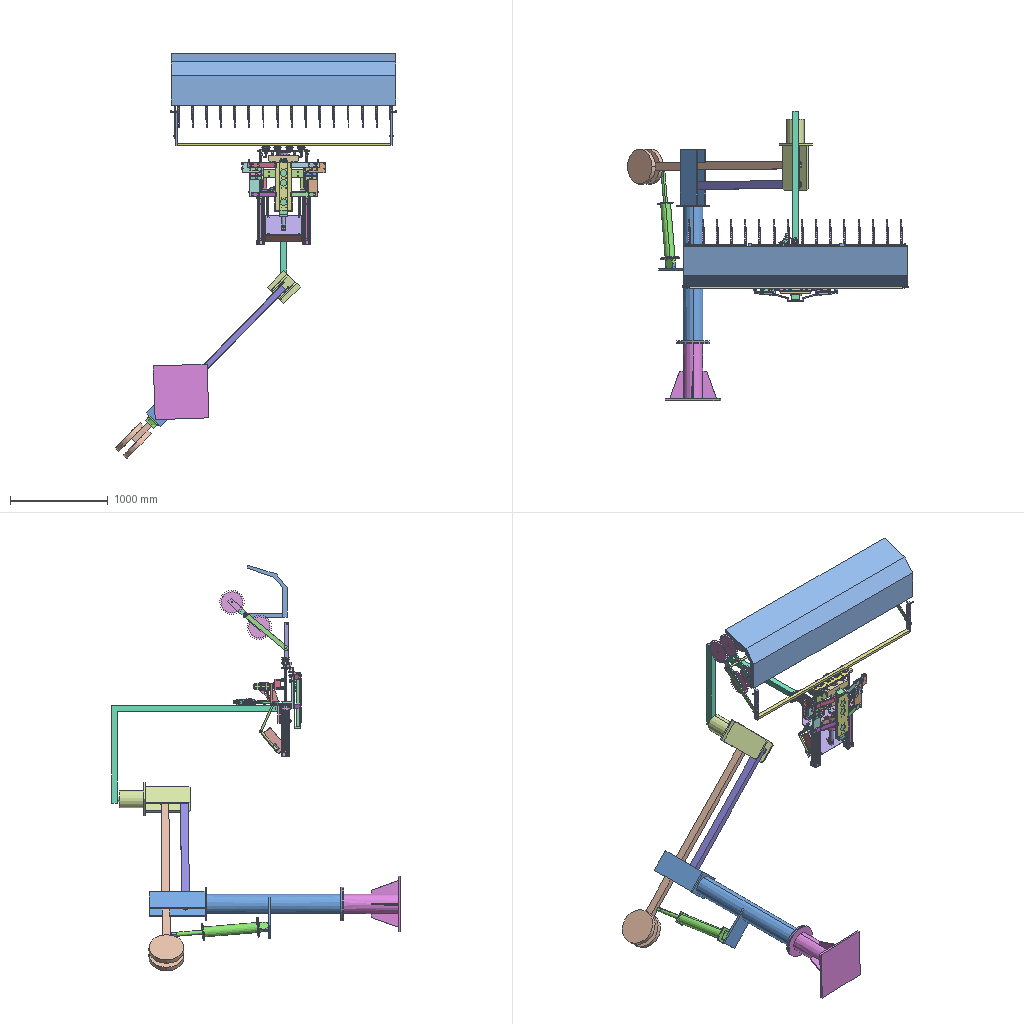Assembly | SolidWorks | 178 different items | 243 placed | box 2879 x 2956 x 4152 mm
Parts list (item | name | quantity | parent item | size | volume | features):
1 | (subassembly) | x1 | - | 2314 x 946.381 x 704.175 mm | 91068773 mm3 | features ReferencePattern 16, CompositeCurve 3, LocalLPattern 1, MirrorCompFeat 1
2 | (subassembly) | x1 | in 1 | 363 x 547.441 x 39 mm | 464108 mm3 | -
3 | (subassembly) | x16 | in 1 | 249.717 x 629.836 x 30 mm | 1063690 mm3 | features CompositeCurve 2
4 | - | x1 | - | 73.887 x 126.864 x 54.9 mm | 162557 mm3 | features BaseBody 1
5 | - | x1 | - | 22.207 x 46.689 x 12 mm | 3091 mm3 | features BaseBody 1
6 | - | x1 | - | 30 x 39 x 30 mm | 13063 mm3 | features BaseBody 1
7 | - | x1 | - | 146 x 156.5 x 60 mm | 309564 mm3 | features BaseBody 1
8 | - | x1 | - | 24.32 x 14.119 x 26.558 mm | 2309 mm3 | features BaseBody 1
9 | - | x1 | - | 22.207 x 46.689 x 12 mm | 3091 mm3 | features BaseBody 1
10 | - | x1 | - | 13.769 x 12.7 x 25.7 mm | 2253 mm3 | features BaseBody 1
11 | - | x1 | - | 9.032 x 9.032 x 8 mm | 229.539 mm3 | features BaseBody 1
12 | - | x1 | - | 80 x 120 x 12 mm | 92320 mm3 | features BaseBody 1
13 | - | x1 | - | 4 x 4.6 x 27 mm | 359.458 mm3 | features BaseBody 1
14 | - | x1 | - | 110 x 80 x 200 mm | 382814 mm3 | features BaseBody 1
15 | - | x1 | - | 110 x 60 x 20 mm | 118905 mm3 | features BaseBody 1
16 | - | x1 | - | 23.075 x 23.71 x 12.8 mm | 3293 mm3 | features BaseBody 1
17 | - | x1 | - | 18.984 x 34.285 x 13 mm | 2185 mm3 | features BaseBody 1
18 | - | x1 | - | 175.5 x 100 x 350 mm | 747572 mm3 | features BaseBody 1
19 | - | x1 | - | 51.292 x 82.808 x 39 mm | 48232 mm3 | features BaseBody 1
20 | - | x1 | - | 22.207 x 46.689 x 12 mm | 3091 mm3 | features BaseBody 1
21 | - | x1 | - | 98.795 x 165.44 x 65 mm | 242429 mm3 | features BaseBody 1
22 | - | x1 | - | 40 x 15 x 88 mm | 34270 mm3 | features BaseBody 1
23 | - | x1 | - | 10.8 x 18 x 20.785 mm | 2106 mm3 | features BaseBody 1
24 | - | x1 | - | 30 x 36 x 30 mm | 8594 mm3 | features BaseBody 1
25 | - | x1 | - | 123 x 40 x 30 mm | 63857 mm3 | features BaseBody 1
26 | - | x1 | - | 15.3 x 33.7 x 33.7 mm | 12419 mm3 | features BaseBody 1
27 | - | x1 | - | 500 x 15 x 80 mm | 587908 mm3 | features BaseBody 1
28 | - | x1 | - | 123 x 40 x 30 mm | 63756 mm3 | features BaseBody 1
29 | - | x1 | - | 4 x 27 x 4.6 mm | 359.458 mm3 | features BaseBody 1
30 | - | x1 | - | 88 x 88 x 34 mm | 174107 mm3 | features BaseBody 1
31 | - | x1 | - | 110 x 12 x 70 mm | 73432 mm3 | features BaseBody 1
32 | - | x1 | - | 30 x 36 x 30 mm | 10896 mm3 | features BaseBody 1
33 | - | x1 | - | 30 x 30 x 60 mm | 22398 mm3 | features BaseBody 1
34 | - | x1 | - | 85.101 x 85.101 x 37 mm | 155072 mm3 | features BaseBody 1
35 | - | x1 | - | 184 x 15 x 184 mm | 494221 mm3 | features BaseBody 1
36 | - | x1 | - | 22.687 x 23.928 x 12.8 mm | 3293 mm3 | features BaseBody 1
37 | - | x1 | - | 13.769 x 12.7 x 25.7 mm | 2253 mm3 | features BaseBody 1
38 | - | x1 | - | 262 x 73 x 50 mm | 166333 mm3 | features BaseBody 1
39 | - | x1 | - | 15.3 x 33.7 x 33.7 mm | 12172 mm3 | features BaseBody 1
40 | - | x1 | - | 262 x 73 x 50 mm | 165869 mm3 | features BaseBody 1
41 | - | x1 | - | 262 x 73 x 50 mm | 167970 mm3 | features BaseBody 1
42 | - | x1 | - | 110 x 80 x 200 mm | 383509 mm3 | features BaseBody 1
43 | - | x1 | - | 22.195 x 25.4 x 6 mm | 1499 mm3 | features BaseBody 1
44 | - | x1 | - | 339.392 x 731.247 x 339.392 mm | 11422226 mm3 | features BaseBody 1
45 | - | x1 | - | 80 x 120 x 12 mm | 91578 mm3 | features BaseBody 1
46 | - | x1 | - | 123 x 40 x 30 mm | 62963 mm3 | features BaseBody 1
47 | - | x1 | - | 27.567 x 25.293 x 10 mm | 3303 mm3 | features BaseBody 1
48 | - | x1 | - | 44 x 40 x 40 mm | 13461 mm3 | features BaseBody 1
49 | - | x1 | - | 123 x 40 x 30 mm | 63542 mm3 | features BaseBody 1
50 | - | x1 | - | 4 x 4.6 x 27 mm | 359.458 mm3 | features BaseBody 1
51 | - | x1 | - | 77 x 77 x 549 mm | 1151888 mm3 | features BaseBody 1
52 | - | x1 | - | 1778 x 360 x 1813 mm | 20939822 mm3 | features BaseBody 1
53 | - | x1 | - | 530 x 100 x 18 mm | 848525 mm3 | features BaseBody 1
54 | - | x1 | - | 36.549 x 18.999 x 35.35 mm | 8339 mm3 | features BaseBody 1
55 | - | x1 | - | 30 x 36 x 30 mm | 10405 mm3 | features BaseBody 1
56 | - | x1 | - | 567.987 x 595 x 567.987 mm | 26013266 mm3 | features BaseBody 1
57 | - | x1 | - | 40 x 15 x 88 mm | 34270 mm3 | features BaseBody 1
58 | - | x1 | - | 44 x 40 x 40 mm | 13461 mm3 | features BaseBody 1
59 | - | x1 | - | 30 x 36 x 30 mm | 10359 mm3 | features BaseBody 1
60 | - | x1 | - | 10.8 x 18 x 20.785 mm | 2106 mm3 | features BaseBody 1
61 | - | x1 | - | 184 x 18 x 184 mm | 496342 mm3 | features BaseBody 1
62 | - | x1 | - | 50 x 166.5 x 50 mm | 64845 mm3 | features BaseBody 1
63 | - | x1 | - | 39.742 x 23.493 x 36.691 mm | 9283 mm3 | features BaseBody 1
64 | - | x1 | - | 144.562 x 43.913 x 64 mm | 15230 mm3 | features BaseBody 1
65 | - | x1 | - | 23.74 x 11.323 x 24 mm | 1594 mm3 | features BaseBody 1
66 | - | x1 | - | 35.811 x 32.932 x 35.35 mm | 8339 mm3 | features BaseBody 1
67 | - | x1 | - | 50 x 83.297 x 85.762 mm | 32586 mm3 | features BaseBody 1
68 | - | x1 | - | 25 x 46.139 x 50 mm | 7662 mm3 | features BaseBody 1
69 | - | x1 | - | 22.207 x 46.689 x 12 mm | 3091 mm3 | features BaseBody 1
70 | - | x1 | - | 30 x 37 x 30 mm | 10515 mm3 | features BaseBody 1
71 | - | x1 | - | 14.343 x 11.893 x 10 mm | 615.272 mm3 | features BaseBody 1
72 | - | x1 | - | 380 x 168.657 x 200.457 mm | 197189 mm3 | features BaseBody 1
73 | - | x1 | - | 18.984 x 34.285 x 13 mm | 2185 mm3 | features BaseBody 1
74 | - | x1 | - | 63 x 63 x 524 mm | 188150 mm3 | features BaseBody 1
75 | - | x1 | - | 22.207 x 46.689 x 12 mm | 3091 mm3 | features BaseBody 1
76 | - | x1 | - | 14.343 x 11.893 x 10 mm | 615.272 mm3 | features BaseBody 1
77 | - | x1 | - | 45 x 45 x 39.5 mm | 21967 mm3 | features BaseBody 1
78 | - | x1 | - | 44 x 40 x 40 mm | 13461 mm3 | features BaseBody 1
79 | - | x2 | in 1 | 18.3 x 18.3 x 25.76 mm | 2486 mm3 | features RevCut 2, ICE 1, LPattern 1, Revolution 1
80 | - | x1 | in 1 | 2300 x 530.953 x 444.384 mm | 70923348 mm3 | features Cut 2, ICE 2, MirrorPattern 1, MoveFace 1, SplitBody 1
81 | - | x16 | in 3 | 50 x 450 x 10 mm | 220288 mm3 | features Extrusion 1
82 | - | x2 | in 1, 2 | 7 x 77.287 x 581.266 mm | 173888 mm3 | features Extrusion 1
83 | - | x1 | - | 15.3 x 33.7 x 33.7 mm | 11915 mm3 | features BaseBody 1
84 | - | x2 | in 1, 2 | 363 x 40 x 20 mm | 288260 mm3 | features Cut 1, Extrusion 1, HoleWzd 1, ICE 1
85 | - | x2 | in 1, 2 | 8 x 8 x 39 mm | 1960 mm3 | features Extrusion 1
86 | - | x1 | in 1 | 25 x 40 x 2181 mm | 2180980 mm3 | features Extrusion 1
87 | - | x32 | in 3 | 249.717 x 249.434 x 10 mm | 421701 mm3 | features Extrusion 1
88 | - | x1 | - | 66 x 184 x 66 mm | 425451 mm3 | features BaseBody 1
89 | - | x1 | - | 262 x 73 x 50 mm | 165745 mm3 | features BaseBody 1
90 | - | x1 | - | 158.743 x 176.419 x 16 mm | 247944 mm3 | features BaseBody 1
91 | - | x1 | - | 24.828 x 24.19 x 6 mm | 1499 mm3 | features BaseBody 1
92 | - | x1 | - | 8 x 6 x 8 mm | 229.539 mm3 | features BaseBody 1
93 | - | x1 | - | 184 x 108 x 57.2 mm | 359196 mm3 | features BaseBody 1
94 | - | x1 | - | 44 x 40 x 40 mm | 13461 mm3 | features BaseBody 1
95 | - | x1 | - | 300 x 125 x 217 mm | 835865 mm3 | features BaseBody 1
96 | - | x1 | - | 45 x 45 x 41.5 mm | 22254 mm3 | features BaseBody 1
97 | - | x1 | - | 175.5 x 100 x 350 mm | 742492 mm3 | features BaseBody 1
98 | - | x1 | - | 44 x 40 x 40 mm | 13461 mm3 | features BaseBody 1
99 | - | x1 | - | 30 x 46 x 30 mm | 10612 mm3 | features BaseBody 1
100 | - | x1 | - | 148 x 94 x 64 mm | 563266 mm3 | features BaseBody 1
101 | - | x1 | - | 63 x 63 x 524 mm | 188170 mm3 | features BaseBody 1
102 | - | x1 | - | 44 x 40 x 40 mm | 13461 mm3 | features BaseBody 1
103 | - | x1 | - | 112 x 23.5 x 44.5 mm | 84873 mm3 | features BaseBody 1
104 | - | x1 | - | 10.8 x 18 x 20.785 mm | 2106 mm3 | features BaseBody 1
105 | - | x1 | - | 45 x 45 x 41.5 mm | 22254 mm3 | features BaseBody 1
106 | - | x1 | - | 160 x 10 x 485 mm | 649264 mm3 | features BaseBody 1
107 | - | x1 | - | 22.195 x 25.4 x 6 mm | 1499 mm3 | features BaseBody 1
108 | - | x1 | - | 260 x 30 x 10 mm | 49540 mm3 | features BaseBody 1
109 | - | x1 | - | 521.246 x 1975 x 525.819 mm | 52229726 mm3 | features BaseBody 1
110 | - | x1 | - | 60 x 1700 x 1049 mm | 9509525 mm3 | features BaseBody 1
111 | - | x1 | - | 24.828 x 24.19 x 6 mm | 1499 mm3 | features BaseBody 1
112 | - | x1 | - | 24.828 x 24.19 x 6 mm | 1499 mm3 | features BaseBody 1
113 | - | x1 | - | 13.769 x 12.7 x 25.7 mm | 2253 mm3 | features BaseBody 1
114 | - | x1 | - | 15.3 x 33.7 x 33.7 mm | 12319 mm3 | features BaseBody 1
115 | - | x1 | - | 1155 x 90.969 x 1178 mm | 7300531 mm3 | features BaseBody 1
116 | - | x1 | - | 85.101 x 85.101 x 37 mm | 155072 mm3 | features BaseBody 1
117 | - | x1 | - | 4 x 27 x 4.6 mm | 359.458 mm3 | features BaseBody 1
118 | - | x1 | - | 72 x 72 x 416.14 mm | 547741 mm3 | features BaseBody 1
119 | - | x1 | - | 4 x 27 x 4.6 mm | 359.458 mm3 | features BaseBody 1
120 | - | x1 | - | 380 x 251.39 x 269.878 mm | 364758 mm3 | features BaseBody 1
121 | - | x1 | - | 50 x 83.297 x 85.762 mm | 32586 mm3 | features BaseBody 1
122 | - | x1 | - | 22.207 x 46.689 x 12 mm | 3091 mm3 | features BaseBody 1
123 | - | x1 | - | 34 x 58.835 x 50.022 mm | 10435 mm3 | features BaseBody 1
124 | - | x1 | - | 22.207 x 46.689 x 12 mm | 3091 mm3 | features BaseBody 1
125 | - | x1 | - | 3.626 x 9.6 x 9.485 mm | 14.041 mm3 | features BaseBody 1
126 | - | x1 | - | 30 x 58.835 x 50.022 mm | 9184 mm3 | features BaseBody 1
127 | - | x1 | - | 4.6 x 4 x 27 mm | 359.458 mm3 | features BaseBody 1
128 | - | x1 | - | 45 x 45 x 41.5 mm | 22254 mm3 | features BaseBody 1
129 | - | x1 | - | 22.195 x 25.4 x 6 mm | 1499 mm3 | features BaseBody 1
130 | - | x1 | - | 230.771 x 990.893 x 231.743 mm | 5798117 mm3 | features BaseBody 1
131 | - | x1 | - | 85.101 x 85.101 x 37 mm | 155072 mm3 | features BaseBody 1
132 | - | x1 | - | 64.24 x 45.879 x 64 mm | 49930 mm3 | features BaseBody 1
133 | - | x1 | - | 110 x 65 x 20 mm | 129905 mm3 | features BaseBody 1
134 | - | x1 | - | 30 x 30 x 65 mm | 25106 mm3 | features BaseBody 1
135 | - | x1 | - | 85.101 x 85.101 x 37 mm | 155072 mm3 | features BaseBody 1
136 | - | x1 | - | 24.828 x 24.19 x 6 mm | 1499 mm3 | features BaseBody 1
137 | - | x1 | - | 8 x 6 x 8 mm | 229.539 mm3 | features BaseBody 1
138 | - | x1 | - | 22.195 x 25.4 x 4 mm | 1001 mm3 | features BaseBody 1
139 | - | x1 | - | 20 x 20 x 85 mm | 21756 mm3 | features BaseBody 1
140 | - | x1 | - | 46.461 x 34.481 x 18.522 mm | 9283 mm3 | features BaseBody 1
141 | - | x1 | - | 22.207 x 46.689 x 12 mm | 3091 mm3 | features BaseBody 1
142 | - | x1 | - | 500 x 15 x 80 mm | 581983 mm3 | features BaseBody 1
143 | - | x1 | - | 9.032 x 9.032 x 8 mm | 229.539 mm3 | features BaseBody 1
144 | - | x1 | - | 34.458 x 52.569 x 26.335 mm | 4644 mm3 | features BaseBody 1
145 | - | x1 | - | 10.8 x 18 x 20.785 mm | 2106 mm3 | features BaseBody 1
146 | - | x1 | - | 10.8 x 18 x 20.785 mm | 2106 mm3 | features BaseBody 1
147 | - | x1 | - | 123 x 40 x 30 mm | 63756 mm3 | features BaseBody 1
148 | - | x1 | - | 15 x 60 x 110 mm | 93137 mm3 | features BaseBody 1
149 | - | x1 | - | 15 x 60 x 110 mm | 93077 mm3 | features BaseBody 1
150 | - | x1 | - | 30 x 36 x 30 mm | 10433 mm3 | features BaseBody 1
151 | - | x1 | - | 15.3 x 33.7 x 33.7 mm | 12319 mm3 | features BaseBody 1
152 | - | x1 | - | 4.6 x 4 x 27 mm | 359.458 mm3 | features BaseBody 1
153 | - | x1 | - | 720 x 215 x 15 mm | 1921061 mm3 | features BaseBody 1
154 | - | x1 | - | 50 x 166.5 x 50 mm | 64845 mm3 | features BaseBody 1
155 | - | x1 | - | 77 x 77 x 549 mm | 1158524 mm3 | features BaseBody 1
156 | - | x1 | - | 86 x 63 x 576 mm | 613007 mm3 | features BaseBody 1
157 | - | x1 | - | 20 x 20 x 85 mm | 21756 mm3 | features BaseBody 1
158 | - | x1 | - | 10.8 x 18 x 20.785 mm | 2106 mm3 | features BaseBody 1
159 | - | x1 | - | 123 x 40 x 30 mm | 63852 mm3 | features BaseBody 1
160 | - | x1 | - | 15.3 x 33.7 x 33.7 mm | 12319 mm3 | features BaseBody 1
161 | - | x1 | - | 100 x 194 x 128 mm | 497627 mm3 | features BaseBody 1
162 | - | x1 | - | 35.811 x 32.932 x 35.35 mm | 8339 mm3 | features BaseBody 1
163 | - | x1 | - | 66 x 184 x 66 mm | 428858 mm3 | features BaseBody 1
164 | - | x1 | - | 110 x 12 x 70 mm | 74267 mm3 | features BaseBody 1
165 | - | x1 | - | 27.569 x 10 x 25.285 mm | 3303 mm3 | features BaseBody 1
166 | - | x1 | - | 184 x 108 x 57.2 mm | 359196 mm3 | features BaseBody 1
167 | - | x1 | - | 25.158 x 10 x 27.599 mm | 3303 mm3 | features BaseBody 1
168 | - | x1 | - | 18.984 x 34.285 x 13 mm | 2185 mm3 | features BaseBody 1
169 | - | x1 | - | 76.059 x 188.139 x 49.5 mm | 95194 mm3 | features BaseBody 1
170 | - | x1 | - | 39.412 x 23.824 x 36.315 mm | 9283 mm3 | features BaseBody 1
171 | - | x1 | - | 18.984 x 34.285 x 13 mm | 2185 mm3 | features BaseBody 1
172 | - | x1 | - | 470.221 x 190.46 x 471.381 mm | 503969 mm3 | features BaseBody 1
173 | - | x1 | - | 3.626 x 9.6 x 9.485 mm | 14.041 mm3 | features BaseBody 1
174 | - | x1 | - | 33.242 x 52.569 x 26.335 mm | 4644 mm3 | features BaseBody 1
175 | - | x1 | - | 27.621 x 25.047 x 10 mm | 3303 mm3 | features BaseBody 1
176 | - | x1 | - | 39.045 x 20.983 x 35.35 mm | 8720 mm3 | features BaseBody 1
177 | - | x1 | - | 4 x 27 x 4.6 mm | 359.458 mm3 | features BaseBody 1
178 | hex bolt gradeab_iso | x1 | - | - | - | -
Mates (type | each side: item.copy, entity, surface, feature):
In the top assembly
Coincident | 131.1 face plane Import 1 | 86.1 face plane Boss-Extrude 1
Coincident | 34.1 face plane Import 1 | 86.1 face plane Boss-Extrude 1
Width | 53.1 face plane Import 1 | 53.1 face plane Import 1 | 86.1 face plane Boss-Extrude 1 | 86.1 face plane Boss-Extrude 1
Width | 84.1 face plane Boss-Extrude 1 | 84.2 face plane Boss-Extrude 1 | 53.1 face plane Import 1 | 53.1 face plane Import 1
In subassembly 1
Concentric | 80.1 face cylinder BasePart-Frame Three Point-1 | 81.1 face cylinder Boss-Extrude 1
Concentric | 80.1 face cylinder Cut-Extrude 2 | 79.1 face cylinder Base-Revolve
Coincident | 80.1 face plane Boss-Extrude 1 | 79.1 face plane Base-Revolve
Parallel | 80.1 face plane BasePart-Frame Three Point-1 | 84.3 face plane Boss-Extrude 1
Concentric | 80.1 face cylinder BasePart-Frame Three Point-1 | 82.1 face cylinder Boss-Extrude 1
DistanceDim | 81.1 face plane Boss-Extrude 1 | 82.1 face plane Boss-Extrude 1
Concentric | 80.1 face cylinder BasePart-Frame Three Point-1 | 82.2 edge
Parallel | 84.4 face plane Boss-Extrude 1 | 84.3 face plane Boss-Extrude 1 | 2 times
Coincident | 84.4 face plane Boss-Extrude 1 | 82.2 face plane Boss-Extrude 1
Concentric | 84.4 face cylinder Boss-Extrude 1 | 82.2 face cylinder Boss-Extrude 1
Concentric | 82.2 face cylinder Boss-Extrude 1 | 85.1 face cylinder Boss-Extrude 1
Coincident | 80.1 edge | 82.2 face plane Boss-Extrude 1
InPlace | 84.4 face plane Boss-Extrude 1 | 86.2 plane
In subassembly 3
Concentric | 87.1 edge | 81.2 face cylinder Boss-Extrude 1
Coincident | 87.1 face plane Boss-Extrude 4 | 81.2 face plane Boss-Extrude 1
Concentric | 81.2 edge | 87.2 face cylinder Boss-Extrude 4 | 2 times
Coincident | 81.2 face plane Boss-Extrude 1 | 87.2 face plane Boss-Extrude 4
In subassembly 2
Coincident | 84.4 face plane Boss-Extrude 1 | 2.1 plane | 2 times
Concentric | 82.2 face cylinder Boss-Extrude 1 | 85.2 face cylinder Boss-Extrude 1
Concentric | 84.4 face cylinder Boss-Extrude 1 | 85.2 face cylinder Boss-Extrude 1